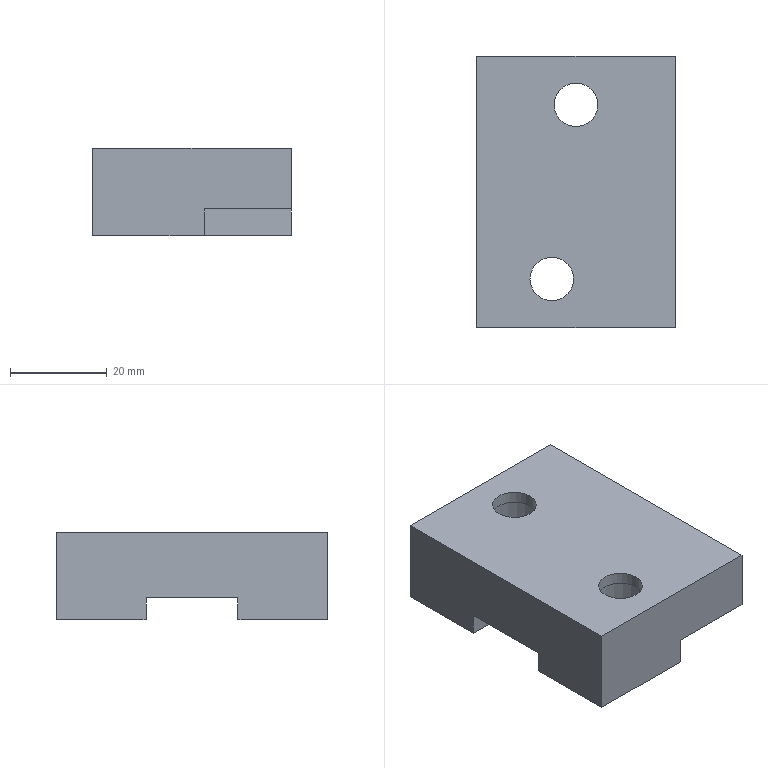Part | STEP file | lll_id2818_x_t | 1 solid | 20 faces | box 41 x 56 x 18 mm | volume 30597 mm3 | plane 16 | cylinder 4 | commonest cylinder face diameters 9.009 x2 14.508 x2
STEP:
#1=CARTESIAN_POINT('',(1546.44,18.,18.));
#2=VERTEX_POINT('',#1);
#3=CARTESIAN_POINT('',(1541.935,18.,18.));
#4=DIRECTION('',(0.,0.,-1.));
#5=DIRECTION('',(1.,0.,0.));
#6=AXIS2_PLACEMENT_3D('',#3,#4,#5);
#7=CIRCLE('',#6,4.505);
#8=EDGE_CURVE('',#2,#2,#7,.T.);
#9=ORIENTED_EDGE('',*,*,#8,.T.);
#10=EDGE_LOOP('',(#9));
#11=FACE_BOUND('',#10,.T.);
#12=CARTESIAN_POINT('',(1562.435,28.,18.));
#13=VERTEX_POINT('',#12);
#14=CARTESIAN_POINT('',(1562.435,-28.,18.));
#15=VERTEX_POINT('',#14);
#16=CARTESIAN_POINT('',(1562.435,0.,18.));
#17=DIRECTION('',(0.,-1.,0.));
#18=VECTOR('',#17,1.);
#19=LINE('',#16,#18);
#20=EDGE_CURVE('',#13,#15,#19,.T.);
#21=ORIENTED_EDGE('',*,*,#20,.F.);
#22=CARTESIAN_POINT('',(1521.435,28.,18.));
#23=VERTEX_POINT('',#22);
#24=CARTESIAN_POINT('',(1531.935,28.,18.));
#25=DIRECTION('',(-1.,0.,0.));
#26=VECTOR('',#25,1.);
#27=LINE('',#24,#26);
#28=EDGE_CURVE('',#13,#23,#27,.T.);
#29=ORIENTED_EDGE('',*,*,#28,.T.);
#30=CARTESIAN_POINT('',(1521.435,-28.,18.));
#31=VERTEX_POINT('',#30);
#32=CARTESIAN_POINT('',(1521.435,0.,18.));
#33=DIRECTION('',(0.,1.,0.));
#34=VECTOR('',#33,1.);
#35=LINE('',#32,#34);
#36=EDGE_CURVE('',#31,#23,#35,.T.);
#37=ORIENTED_EDGE('',*,*,#36,.F.);
#38=CARTESIAN_POINT('',(1531.935,-28.,18.));
#39=DIRECTION('',(-1.,0.,0.));
#40=VECTOR('',#39,1.);
#41=LINE('',#38,#40);
#42=EDGE_CURVE('',#15,#31,#41,.T.);
#43=ORIENTED_EDGE('',*,*,#42,.F.);
#44=EDGE_LOOP('',(#21,#29,#37,#43));
#45=FACE_BOUND('',#44,.T.);
#46=CARTESIAN_POINT('',(1541.44,-18.,18.));
#47=VERTEX_POINT('',#46);
#48=CARTESIAN_POINT('',(1536.935,-18.,18.));
#49=DIRECTION('',(0.,0.,-1.));
#50=DIRECTION('',(1.,0.,0.));
#51=AXIS2_PLACEMENT_3D('',#48,#49,#50);
#52=CIRCLE('',#51,4.505);
#53=EDGE_CURVE('',#47,#47,#52,.T.);
#54=ORIENTED_EDGE('',*,*,#53,.T.);
#55=EDGE_LOOP('',(#54));
#56=FACE_BOUND('',#55,.T.);
#57=CARTESIAN_POINT('',(1531.935,0.,18.));
#58=DIRECTION('',(0.,0.,1.));
#59=DIRECTION('',(1.,0.,0.));
#60=AXIS2_PLACEMENT_3D('',#57,#58,#59);
#61=PLANE('',#60);
#62=ADVANCED_FACE('',(#11,#45,#56),#61,.T.);
#63=CARTESIAN_POINT('',(1521.435,-9.5,0.));
#64=VERTEX_POINT('',#63);
#65=CARTESIAN_POINT('',(1521.435,-9.5,4.5));
#66=VERTEX_POINT('',#65);
#67=CARTESIAN_POINT('',(1521.435,-9.5,0.));
#68=DIRECTION('',(0.,0.,1.));
#69=VECTOR('',#68,1.);
#70=LINE('',#67,#69);
#71=EDGE_CURVE('',#64,#66,#70,.T.);
#72=ORIENTED_EDGE('',*,*,#71,.T.);
#73=CARTESIAN_POINT('',(1562.435,-9.5,4.5));
#74=VERTEX_POINT('',#73);
#75=CARTESIAN_POINT('',(1594.5,-9.5,4.5));
#76=DIRECTION('',(1.,0.,0.));
#77=VECTOR('',#76,1.);
#78=LINE('',#75,#77);
#79=EDGE_CURVE('',#66,#74,#78,.T.);
#80=ORIENTED_EDGE('',*,*,#79,.T.);
#81=CARTESIAN_POINT('',(1562.435,-9.5,0.));
#82=VERTEX_POINT('',#81);
#83=CARTESIAN_POINT('',(1562.435,-9.5,0.));
#84=DIRECTION('',(0.,0.,-1.));
#85=VECTOR('',#84,1.);
#86=LINE('',#83,#85);
#87=EDGE_CURVE('',#74,#82,#86,.T.);
#88=ORIENTED_EDGE('',*,*,#87,.T.);
#89=CARTESIAN_POINT('',(1531.935,-9.5,0.));
#90=DIRECTION('',(-1.,0.,0.));
#91=VECTOR('',#90,1.);
#92=LINE('',#89,#91);
#93=EDGE_CURVE('',#82,#64,#92,.T.);
#94=ORIENTED_EDGE('',*,*,#93,.T.);
#95=EDGE_LOOP('',(#72,#80,#88,#94));
#96=FACE_OUTER_BOUND('',#95,.T.);
#97=CARTESIAN_POINT('',(1594.5,-9.5,2.5));
#98=DIRECTION('',(0.,-1.,0.));
#99=DIRECTION('',(0.,0.,-1.));
#100=AXIS2_PLACEMENT_3D('',#97,#98,#99);
#101=PLANE('',#100);
#102=ADVANCED_FACE('',(#96),#101,.F.);
#103=CARTESIAN_POINT('',(1521.435,9.5,4.5));
#104=VERTEX_POINT('',#103);
#105=CARTESIAN_POINT('',(1521.435,0.,4.5));
#106=DIRECTION('',(0.,-1.,0.));
#107=VECTOR('',#106,1.);
#108=LINE('',#105,#107);
#109=EDGE_CURVE('',#104,#66,#108,.T.);
#110=ORIENTED_EDGE('',*,*,#109,.F.);
#111=CARTESIAN_POINT('',(1562.435,9.5,4.5));
#112=VERTEX_POINT('',#111);
#113=CARTESIAN_POINT('',(1594.5,9.5,4.5));
#114=DIRECTION('',(1.,0.,0.));
#115=VECTOR('',#114,1.);
#116=LINE('',#113,#115);
#117=EDGE_CURVE('',#104,#112,#116,.T.);
#118=ORIENTED_EDGE('',*,*,#117,.T.);
#119=CARTESIAN_POINT('',(1562.435,0.,4.5));
#120=DIRECTION('',(0.,1.,0.));
#121=VECTOR('',#120,1.);
#122=LINE('',#119,#121);
#123=EDGE_CURVE('',#74,#112,#122,.T.);
#124=ORIENTED_EDGE('',*,*,#123,.F.);
#125=ORIENTED_EDGE('',*,*,#79,.F.);
#126=EDGE_LOOP('',(#110,#118,#124,#125));
#127=FACE_OUTER_BOUND('',#126,.T.);
#128=CARTESIAN_POINT('',(12281.383,-13712.786,4.5));
#129=DIRECTION('',(0.,0.,-1.));
#130=DIRECTION('',(-1.,0.,0.));
#131=AXIS2_PLACEMENT_3D('',#128,#129,#130);
#132=PLANE('',#131);
#133=ADVANCED_FACE('',(#127),#132,.T.);
#134=CARTESIAN_POINT('',(1521.435,9.5,0.));
#135=VERTEX_POINT('',#134);
#136=CARTESIAN_POINT('',(1521.435,9.5,2.5));
#137=DIRECTION('',(0.,0.,1.));
#138=VECTOR('',#137,1.);
#139=LINE('',#136,#138);
#140=EDGE_CURVE('',#135,#104,#139,.T.);
#141=ORIENTED_EDGE('',*,*,#140,.F.);
#142=CARTESIAN_POINT('',(1562.435,9.5,0.));
#143=VERTEX_POINT('',#142);
#144=CARTESIAN_POINT('',(1531.935,9.5,0.));
#145=DIRECTION('',(-1.,0.,0.));
#146=VECTOR('',#145,1.);
#147=LINE('',#144,#146);
#148=EDGE_CURVE('',#143,#135,#147,.T.);
#149=ORIENTED_EDGE('',*,*,#148,.F.);
#150=CARTESIAN_POINT('',(1562.435,9.5,2.5));
#151=DIRECTION('',(0.,0.,-1.));
#152=VECTOR('',#151,1.);
#153=LINE('',#150,#152);
#154=EDGE_CURVE('',#112,#143,#153,.T.);
#155=ORIENTED_EDGE('',*,*,#154,.F.);
#156=ORIENTED_EDGE('',*,*,#117,.F.);
#157=EDGE_LOOP('',(#141,#149,#155,#156));
#158=FACE_OUTER_BOUND('',#157,.T.);
#159=CARTESIAN_POINT('',(1594.5,9.5,2.5));
#160=DIRECTION('',(0.,1.,0.));
#161=DIRECTION('',(0.,0.,-1.));
#162=AXIS2_PLACEMENT_3D('',#159,#160,#161);
#163=PLANE('',#162);
#164=ADVANCED_FACE('',(#158),#163,.F.);
#165=CARTESIAN_POINT('',(1521.435,28.,0.));
#166=VERTEX_POINT('',#165);
#167=CARTESIAN_POINT('',(1521.435,28.,0.));
#168=DIRECTION('',(0.,0.,1.));
#169=VECTOR('',#168,1.);
#170=LINE('',#167,#169);
#171=EDGE_CURVE('',#166,#23,#170,.T.);
#172=ORIENTED_EDGE('',*,*,#171,.T.);
#173=ORIENTED_EDGE('',*,*,#28,.F.);
#174=CARTESIAN_POINT('',(1562.435,28.,5.5));
#175=VERTEX_POINT('',#174);
#176=CARTESIAN_POINT('',(1562.435,28.,0.));
#177=DIRECTION('',(0.,0.,1.));
#178=VECTOR('',#177,1.);
#179=LINE('',#176,#178);
#180=EDGE_CURVE('',#175,#13,#179,.T.);
#181=ORIENTED_EDGE('',*,*,#180,.F.);
#182=CARTESIAN_POINT('',(1544.435,28.,5.5));
#183=VERTEX_POINT('',#182);
#184=CARTESIAN_POINT('',(1531.935,28.,5.5));
#185=DIRECTION('',(-1.,0.,0.));
#186=VECTOR('',#185,1.);
#187=LINE('',#184,#186);
#188=EDGE_CURVE('',#175,#183,#187,.T.);
#189=ORIENTED_EDGE('',*,*,#188,.T.);
#190=CARTESIAN_POINT('',(1544.435,28.,0.));
#191=VERTEX_POINT('',#190);
#192=CARTESIAN_POINT('',(1544.435,28.,0.));
#193=DIRECTION('',(0.,0.,-1.));
#194=VECTOR('',#193,1.);
#195=LINE('',#192,#194);
#196=EDGE_CURVE('',#183,#191,#195,.T.);
#197=ORIENTED_EDGE('',*,*,#196,.T.);
#198=CARTESIAN_POINT('',(1531.935,28.,0.));
#199=DIRECTION('',(1.,0.,0.));
#200=VECTOR('',#199,1.);
#201=LINE('',#198,#200);
#202=EDGE_CURVE('',#166,#191,#201,.T.);
#203=ORIENTED_EDGE('',*,*,#202,.F.);
#204=EDGE_LOOP('',(#172,#173,#181,#189,#197,#203));
#205=FACE_OUTER_BOUND('',#204,.T.);
#206=CARTESIAN_POINT('',(1531.935,28.,0.));
#207=DIRECTION('',(0.,1.,0.));
#208=DIRECTION('',(0.,0.,-1.));
#209=AXIS2_PLACEMENT_3D('',#206,#207,#208);
#210=PLANE('',#209);
#211=ADVANCED_FACE('',(#205),#210,.T.);
#212=CARTESIAN_POINT('',(1521.435,-28.,0.));
#213=VERTEX_POINT('',#212);
#214=CARTESIAN_POINT('',(1521.435,-28.,0.));
#215=DIRECTION('',(0.,0.,1.));
#216=VECTOR('',#215,1.);
#217=LINE('',#214,#216);
#218=EDGE_CURVE('',#213,#31,#217,.T.);
#219=ORIENTED_EDGE('',*,*,#218,.T.);
#220=ORIENTED_EDGE('',*,*,#36,.T.);
#221=ORIENTED_EDGE('',*,*,#171,.F.);
#222=CARTESIAN_POINT('',(1521.435,0.,0.));
#223=DIRECTION('',(0.,1.,0.));
#224=VECTOR('',#223,1.);
#225=LINE('',#222,#224);
#226=EDGE_CURVE('',#135,#166,#225,.T.);
#227=ORIENTED_EDGE('',*,*,#226,.F.);
#228=ORIENTED_EDGE('',*,*,#140,.T.);
#229=ORIENTED_EDGE('',*,*,#109,.T.);
#230=ORIENTED_EDGE('',*,*,#71,.F.);
#231=CARTESIAN_POINT('',(1521.435,0.,0.));
#232=DIRECTION('',(0.,-1.,0.));
#233=VECTOR('',#232,1.);
#234=LINE('',#231,#233);
#235=EDGE_CURVE('',#64,#213,#234,.T.);
#236=ORIENTED_EDGE('',*,*,#235,.T.);
#237=EDGE_LOOP('',(#219,#220,#221,#227,#228,#229,#230,#236));
#238=FACE_OUTER_BOUND('',#237,.T.);
#239=CARTESIAN_POINT('',(1521.435,0.,0.));
#240=DIRECTION('',(-1.,0.,0.));
#241=DIRECTION('',(0.,0.,1.));
#242=AXIS2_PLACEMENT_3D('',#239,#240,#241);
#243=PLANE('',#242);
#244=ADVANCED_FACE('',(#238),#243,.T.);
#245=CARTESIAN_POINT('',(1562.435,10.,0.));
#246=VERTEX_POINT('',#245);
#247=CARTESIAN_POINT('',(1562.435,10.,5.5));
#248=VERTEX_POINT('',#247);
#249=CARTESIAN_POINT('',(1562.435,10.,0.));
#250=DIRECTION('',(0.,0.,1.));
#251=VECTOR('',#250,1.);
#252=LINE('',#249,#251);
#253=EDGE_CURVE('',#246,#248,#252,.T.);
#254=ORIENTED_EDGE('',*,*,#253,.T.);
#255=CARTESIAN_POINT('',(1562.435,0.,5.5));
#256=DIRECTION('',(0.,-1.,0.));
#257=VECTOR('',#256,1.);
#258=LINE('',#255,#257);
#259=EDGE_CURVE('',#175,#248,#258,.T.);
#260=ORIENTED_EDGE('',*,*,#259,.F.);
#261=ORIENTED_EDGE('',*,*,#180,.T.);
#262=ORIENTED_EDGE('',*,*,#20,.T.);
#263=CARTESIAN_POINT('',(1562.435,-28.,5.5));
#264=VERTEX_POINT('',#263);
#265=CARTESIAN_POINT('',(1562.435,-28.,0.));
#266=DIRECTION('',(0.,0.,1.));
#267=VECTOR('',#266,1.);
#268=LINE('',#265,#267);
#269=EDGE_CURVE('',#264,#15,#268,.T.);
#270=ORIENTED_EDGE('',*,*,#269,.F.);
#271=CARTESIAN_POINT('',(1562.435,-10.,5.5));
#272=VERTEX_POINT('',#271);
#273=CARTESIAN_POINT('',(1562.435,0.,5.5));
#274=DIRECTION('',(0.,-1.,0.));
#275=VECTOR('',#274,1.);
#276=LINE('',#273,#275);
#277=EDGE_CURVE('',#272,#264,#276,.T.);
#278=ORIENTED_EDGE('',*,*,#277,.F.);
#279=CARTESIAN_POINT('',(1562.435,-10.,0.));
#280=VERTEX_POINT('',#279);
#281=CARTESIAN_POINT('',(1562.435,-10.,0.));
#282=DIRECTION('',(0.,0.,-1.));
#283=VECTOR('',#282,1.);
#284=LINE('',#281,#283);
#285=EDGE_CURVE('',#272,#280,#284,.T.);
#286=ORIENTED_EDGE('',*,*,#285,.T.);
#287=CARTESIAN_POINT('',(1562.435,0.,0.));
#288=DIRECTION('',(0.,1.,0.));
#289=VECTOR('',#288,1.);
#290=LINE('',#287,#289);
#291=EDGE_CURVE('',#280,#82,#290,.T.);
#292=ORIENTED_EDGE('',*,*,#291,.T.);
#293=ORIENTED_EDGE('',*,*,#87,.F.);
#294=ORIENTED_EDGE('',*,*,#123,.T.);
#295=ORIENTED_EDGE('',*,*,#154,.T.);
#296=CARTESIAN_POINT('',(1562.435,0.,0.));
#297=DIRECTION('',(0.,-1.,0.));
#298=VECTOR('',#297,1.);
#299=LINE('',#296,#298);
#300=EDGE_CURVE('',#246,#143,#299,.T.);
#301=ORIENTED_EDGE('',*,*,#300,.F.);
#302=EDGE_LOOP('',(#254,#260,#261,#262,#270,#278,#286,#292,#293,#294,#295,#301));
#303=FACE_OUTER_BOUND('',#302,.T.);
#304=CARTESIAN_POINT('',(1562.435,0.,0.));
#305=DIRECTION('',(1.,0.,0.));
#306=DIRECTION('',(0.,0.,-1.));
#307=AXIS2_PLACEMENT_3D('',#304,#305,#306);
#308=PLANE('',#307);
#309=ADVANCED_FACE('',(#303),#308,.T.);
#310=CARTESIAN_POINT('',(1544.435,-28.,0.));
#311=VERTEX_POINT('',#310);
#312=CARTESIAN_POINT('',(1531.935,-28.,0.));
#313=DIRECTION('',(1.,0.,0.));
#314=VECTOR('',#313,1.);
#315=LINE('',#312,#314);
#316=EDGE_CURVE('',#213,#311,#315,.T.);
#317=ORIENTED_EDGE('',*,*,#316,.T.);
#318=CARTESIAN_POINT('',(1544.435,-28.,5.5));
#319=VERTEX_POINT('',#318);
#320=CARTESIAN_POINT('',(1544.435,-28.,0.));
#321=DIRECTION('',(0.,0.,1.));
#322=VECTOR('',#321,1.);
#323=LINE('',#320,#322);
#324=EDGE_CURVE('',#311,#319,#323,.T.);
#325=ORIENTED_EDGE('',*,*,#324,.T.);
#326=CARTESIAN_POINT('',(1531.935,-28.,5.5));
#327=DIRECTION('',(1.,0.,0.));
#328=VECTOR('',#327,1.);
#329=LINE('',#326,#328);
#330=EDGE_CURVE('',#319,#264,#329,.T.);
#331=ORIENTED_EDGE('',*,*,#330,.T.);
#332=ORIENTED_EDGE('',*,*,#269,.T.);
#333=ORIENTED_EDGE('',*,*,#42,.T.);
#334=ORIENTED_EDGE('',*,*,#218,.F.);
#335=EDGE_LOOP('',(#317,#325,#331,#332,#333,#334));
#336=FACE_OUTER_BOUND('',#335,.T.);
#337=CARTESIAN_POINT('',(1531.935,-28.,0.));
#338=DIRECTION('',(0.,-1.,0.));
#339=DIRECTION('',(0.,0.,-1.));
#340=AXIS2_PLACEMENT_3D('',#337,#338,#339);
#341=PLANE('',#340);
#342=ADVANCED_FACE('',(#336),#341,.T.);
#343=CARTESIAN_POINT('',(1534.681,18.,0.));
#344=VERTEX_POINT('',#343);
#345=CARTESIAN_POINT('',(1541.935,18.,0.));
#346=DIRECTION('',(0.,0.,-1.));
#347=DIRECTION('',(-1.,0.,0.));
#348=AXIS2_PLACEMENT_3D('',#345,#346,#347);
#349=CIRCLE('',#348,7.254);
#350=EDGE_CURVE('',#344,#344,#349,.T.);
#351=ORIENTED_EDGE('',*,*,#350,.F.);
#352=EDGE_LOOP('',(#351));
#353=FACE_BOUND('',#352,.T.);
#354=ORIENTED_EDGE('',*,*,#202,.T.);
#355=CARTESIAN_POINT('',(1552.185,20.25,0.));
#356=DIRECTION('',(0.7071,-0.7071,0.));
#357=VECTOR('',#356,1.);
#358=LINE('',#355,#357);
#359=EDGE_CURVE('',#191,#246,#358,.T.);
#360=ORIENTED_EDGE('',*,*,#359,.T.);
#361=ORIENTED_EDGE('',*,*,#300,.T.);
#362=ORIENTED_EDGE('',*,*,#148,.T.);
#363=ORIENTED_EDGE('',*,*,#226,.T.);
#364=EDGE_LOOP('',(#354,#360,#361,#362,#363));
#365=FACE_BOUND('',#364,.T.);
#366=CARTESIAN_POINT('',(1531.935,0.,0.));
#367=DIRECTION('',(0.,0.,-1.));
#368=DIRECTION('',(-1.,0.,0.));
#369=AXIS2_PLACEMENT_3D('',#366,#367,#368);
#370=PLANE('',#369);
#371=ADVANCED_FACE('',(#353,#365),#370,.T.);
#372=CARTESIAN_POINT('',(1529.681,-18.,0.));
#373=VERTEX_POINT('',#372);
#374=CARTESIAN_POINT('',(1536.935,-18.,0.));
#375=DIRECTION('',(0.,0.,-1.));
#376=DIRECTION('',(-1.,0.,0.));
#377=AXIS2_PLACEMENT_3D('',#374,#375,#376);
#378=CIRCLE('',#377,7.254);
#379=EDGE_CURVE('',#373,#373,#378,.T.);
#380=ORIENTED_EDGE('',*,*,#379,.F.);
#381=EDGE_LOOP('',(#380));
#382=FACE_BOUND('',#381,.T.);
#383=ORIENTED_EDGE('',*,*,#291,.F.);
#384=CARTESIAN_POINT('',(1552.185,-20.25,0.));
#385=DIRECTION('',(-0.7071,-0.7071,0.));
#386=VECTOR('',#385,1.);
#387=LINE('',#384,#386);
#388=EDGE_CURVE('',#280,#311,#387,.T.);
#389=ORIENTED_EDGE('',*,*,#388,.T.);
#390=ORIENTED_EDGE('',*,*,#316,.F.);
#391=ORIENTED_EDGE('',*,*,#235,.F.);
#392=ORIENTED_EDGE('',*,*,#93,.F.);
#393=EDGE_LOOP('',(#383,#389,#390,#391,#392));
#394=FACE_BOUND('',#393,.T.);
#395=CARTESIAN_POINT('',(1531.935,0.,0.));
#396=DIRECTION('',(0.,0.,-1.));
#397=DIRECTION('',(-1.,0.,0.));
#398=AXIS2_PLACEMENT_3D('',#395,#396,#397);
#399=PLANE('',#398);
#400=ADVANCED_FACE('',(#382,#394),#399,.T.);
#401=ORIENTED_EDGE('',*,*,#388,.F.);
#402=ORIENTED_EDGE('',*,*,#285,.F.);
#403=CARTESIAN_POINT('',(1544.435,-28.,5.5));
#404=DIRECTION('',(0.7071,0.7071,0.));
#405=VECTOR('',#404,1.);
#406=LINE('',#403,#405);
#407=EDGE_CURVE('',#319,#272,#406,.T.);
#408=ORIENTED_EDGE('',*,*,#407,.F.);
#409=ORIENTED_EDGE('',*,*,#324,.F.);
#410=EDGE_LOOP('',(#401,#402,#408,#409));
#411=FACE_OUTER_BOUND('',#410,.T.);
#412=CARTESIAN_POINT('',(1544.435,-28.,0.));
#413=DIRECTION('',(-0.7071,0.7071,0.));
#414=DIRECTION('',(0.,0.,-1.));
#415=AXIS2_PLACEMENT_3D('',#412,#413,#414);
#416=PLANE('',#415);
#417=ADVANCED_FACE('',(#411),#416,.F.);
#418=ORIENTED_EDGE('',*,*,#359,.F.);
#419=ORIENTED_EDGE('',*,*,#196,.F.);
#420=CARTESIAN_POINT('',(1562.435,10.,5.5));
#421=DIRECTION('',(-0.7071,0.7071,0.));
#422=VECTOR('',#421,1.);
#423=LINE('',#420,#422);
#424=EDGE_CURVE('',#248,#183,#423,.T.);
#425=ORIENTED_EDGE('',*,*,#424,.F.);
#426=ORIENTED_EDGE('',*,*,#253,.F.);
#427=EDGE_LOOP('',(#418,#419,#425,#426));
#428=FACE_OUTER_BOUND('',#427,.T.);
#429=CARTESIAN_POINT('',(1562.435,10.,0.));
#430=DIRECTION('',(-0.7071,-0.7071,0.));
#431=DIRECTION('',(0.,0.,-1.));
#432=AXIS2_PLACEMENT_3D('',#429,#430,#431);
#433=PLANE('',#432);
#434=ADVANCED_FACE('',(#428),#433,.F.);
#435=ORIENTED_EDGE('',*,*,#330,.F.);
#436=ORIENTED_EDGE('',*,*,#407,.T.);
#437=ORIENTED_EDGE('',*,*,#277,.T.);
#438=EDGE_LOOP('',(#435,#436,#437));
#439=FACE_OUTER_BOUND('',#438,.T.);
#440=CARTESIAN_POINT('',(882.435,0.,5.5));
#441=DIRECTION('',(0.,0.,-1.));
#442=DIRECTION('',(1.,0.,0.));
#443=AXIS2_PLACEMENT_3D('',#440,#441,#442);
#444=PLANE('',#443);
#445=ADVANCED_FACE('',(#439),#444,.T.);
#446=ORIENTED_EDGE('',*,*,#259,.T.);
#447=ORIENTED_EDGE('',*,*,#424,.T.);
#448=ORIENTED_EDGE('',*,*,#188,.F.);
#449=EDGE_LOOP('',(#446,#447,#448));
#450=FACE_OUTER_BOUND('',#449,.T.);
#451=CARTESIAN_POINT('',(882.435,0.,5.5));
#452=DIRECTION('',(0.,0.,-1.));
#453=DIRECTION('',(1.,0.,0.));
#454=AXIS2_PLACEMENT_3D('',#451,#452,#453);
#455=PLANE('',#454);
#456=ADVANCED_FACE('',(#450),#455,.T.);
#457=CARTESIAN_POINT('',(1546.44,18.,15.5));
#458=VERTEX_POINT('',#457);
#459=CARTESIAN_POINT('',(1541.935,18.,15.5));
#460=DIRECTION('',(0.,0.,1.));
#461=DIRECTION('',(1.,0.,0.));
#462=AXIS2_PLACEMENT_3D('',#459,#460,#461);
#463=CIRCLE('',#462,4.505);
#464=EDGE_CURVE('',#458,#458,#463,.T.);
#465=ORIENTED_EDGE('',*,*,#464,.F.);
#466=EDGE_LOOP('',(#465));
#467=FACE_BOUND('',#466,.T.);
#468=ORIENTED_EDGE('',*,*,#8,.F.);
#469=EDGE_LOOP('',(#468));
#470=FACE_BOUND('',#469,.T.);
#471=CARTESIAN_POINT('',(1541.935,18.,4.5));
#472=DIRECTION('',(0.,0.,1.));
#473=DIRECTION('',(-1.,0.,0.));
#474=AXIS2_PLACEMENT_3D('',#471,#472,#473);
#475=CYLINDRICAL_SURFACE('',#474,4.505);
#476=ADVANCED_FACE('',(#467,#470),#475,.F.);
#477=ORIENTED_EDGE('',*,*,#464,.T.);
#478=EDGE_LOOP('',(#477));
#479=FACE_BOUND('',#478,.T.);
#480=CARTESIAN_POINT('',(1549.189,18.,15.5));
#481=VERTEX_POINT('',#480);
#482=CARTESIAN_POINT('',(1541.935,18.,15.5));
#483=DIRECTION('',(0.,0.,1.));
#484=DIRECTION('',(1.,0.,0.));
#485=AXIS2_PLACEMENT_3D('',#482,#483,#484);
#486=CIRCLE('',#485,7.254);
#487=EDGE_CURVE('',#481,#481,#486,.T.);
#488=ORIENTED_EDGE('',*,*,#487,.F.);
#489=EDGE_LOOP('',(#488));
#490=FACE_BOUND('',#489,.T.);
#491=CARTESIAN_POINT('',(1541.935,18.,15.5));
#492=DIRECTION('',(0.,0.,1.));
#493=DIRECTION('',(-1.,0.,0.));
#494=AXIS2_PLACEMENT_3D('',#491,#492,#493);
#495=PLANE('',#494);
#496=ADVANCED_FACE('',(#479,#490),#495,.F.);
#497=ORIENTED_EDGE('',*,*,#350,.T.);
#498=EDGE_LOOP('',(#497));
#499=FACE_BOUND('',#498,.T.);
#500=ORIENTED_EDGE('',*,*,#487,.T.);
#501=EDGE_LOOP('',(#500));
#502=FACE_BOUND('',#501,.T.);
#503=CARTESIAN_POINT('',(1541.935,18.,4.5));
#504=DIRECTION('',(0.,0.,1.));
#505=DIRECTION('',(-1.,0.,0.));
#506=AXIS2_PLACEMENT_3D('',#503,#504,#505);
#507=CYLINDRICAL_SURFACE('',#506,7.254);
#508=ADVANCED_FACE('',(#499,#502),#507,.F.);
#509=CARTESIAN_POINT('',(1541.44,-18.,15.5));
#510=VERTEX_POINT('',#509);
#511=CARTESIAN_POINT('',(1536.935,-18.,15.5));
#512=DIRECTION('',(0.,0.,1.));
#513=DIRECTION('',(1.,0.,0.));
#514=AXIS2_PLACEMENT_3D('',#511,#512,#513);
#515=CIRCLE('',#514,4.505);
#516=EDGE_CURVE('',#510,#510,#515,.T.);
#517=ORIENTED_EDGE('',*,*,#516,.F.);
#518=EDGE_LOOP('',(#517));
#519=FACE_BOUND('',#518,.T.);
#520=ORIENTED_EDGE('',*,*,#53,.F.);
#521=EDGE_LOOP('',(#520));
#522=FACE_BOUND('',#521,.T.);
#523=CARTESIAN_POINT('',(1536.935,-18.,4.5));
#524=DIRECTION('',(0.,0.,1.));
#525=DIRECTION('',(-1.,0.,0.));
#526=AXIS2_PLACEMENT_3D('',#523,#524,#525);
#527=CYLINDRICAL_SURFACE('',#526,4.505);
#528=ADVANCED_FACE('',(#519,#522),#527,.F.);
#529=ORIENTED_EDGE('',*,*,#516,.T.);
#530=EDGE_LOOP('',(#529));
#531=FACE_BOUND('',#530,.T.);
#532=CARTESIAN_POINT('',(1544.189,-18.,15.5));
#533=VERTEX_POINT('',#532);
#534=CARTESIAN_POINT('',(1536.935,-18.,15.5));
#535=DIRECTION('',(0.,0.,1.));
#536=DIRECTION('',(1.,0.,0.));
#537=AXIS2_PLACEMENT_3D('',#534,#535,#536);
#538=CIRCLE('',#537,7.254);
#539=EDGE_CURVE('',#533,#533,#538,.T.);
#540=ORIENTED_EDGE('',*,*,#539,.F.);
#541=EDGE_LOOP('',(#540));
#542=FACE_BOUND('',#541,.T.);
#543=CARTESIAN_POINT('',(1536.935,-18.,15.5));
#544=DIRECTION('',(0.,0.,1.));
#545=DIRECTION('',(-1.,0.,0.));
#546=AXIS2_PLACEMENT_3D('',#543,#544,#545);
#547=PLANE('',#546);
#548=ADVANCED_FACE('',(#531,#542),#547,.F.);
#549=ORIENTED_EDGE('',*,*,#379,.T.);
#550=EDGE_LOOP('',(#549));
#551=FACE_BOUND('',#550,.T.);
#552=ORIENTED_EDGE('',*,*,#539,.T.);
#553=EDGE_LOOP('',(#552));
#554=FACE_BOUND('',#553,.T.);
#555=CARTESIAN_POINT('',(1536.935,-18.,4.5));
#556=DIRECTION('',(0.,0.,1.));
#557=DIRECTION('',(-1.,0.,0.));
#558=AXIS2_PLACEMENT_3D('',#555,#556,#557);
#559=CYLINDRICAL_SURFACE('',#558,7.254);
#560=ADVANCED_FACE('',(#551,#554),#559,.F.);
#561=CLOSED_SHELL('',(#62,#102,#133,#164,#211,#244,#309,#342,#371,#400,#417,#434,#445,#456,#476,#496,#508,#528,#548,#560));
#562=MANIFOLD_SOLID_BREP('',#561);
#563=(LENGTH_UNIT()NAMED_UNIT(*)SI_UNIT(.MILLI.,.METRE.));
#564=UNCERTAINTY_MEASURE_WITH_UNIT(LENGTH_MEASURE(0.00002),#563,'','');
#565=(NAMED_UNIT(*)PLANE_ANGLE_UNIT()SI_UNIT($,.RADIAN.));
#566=PLANE_ANGLE_MEASURE_WITH_UNIT(PLANE_ANGLE_MEASURE(0.01745),#565);
#567=DIMENSIONAL_EXPONENTS(0.,0.,0.,0.,0.,0.,0.);
#568=(CONVERSION_BASED_UNIT('DEGREE',#566)NAMED_UNIT(#567)PLANE_ANGLE_UNIT());
#569=(NAMED_UNIT(*)SI_UNIT($,.STERADIAN.)SOLID_ANGLE_UNIT());
#570=(GEOMETRIC_REPRESENTATION_CONTEXT(3)GLOBAL_UNCERTAINTY_ASSIGNED_CONTEXT((#564))GLOBAL_UNIT_ASSIGNED_CONTEXT((#563,#568,#569))REPRESENTATION_CONTEXT('',''));
#571=ADVANCED_BREP_SHAPE_REPRESENTATION('',(#562),#570);